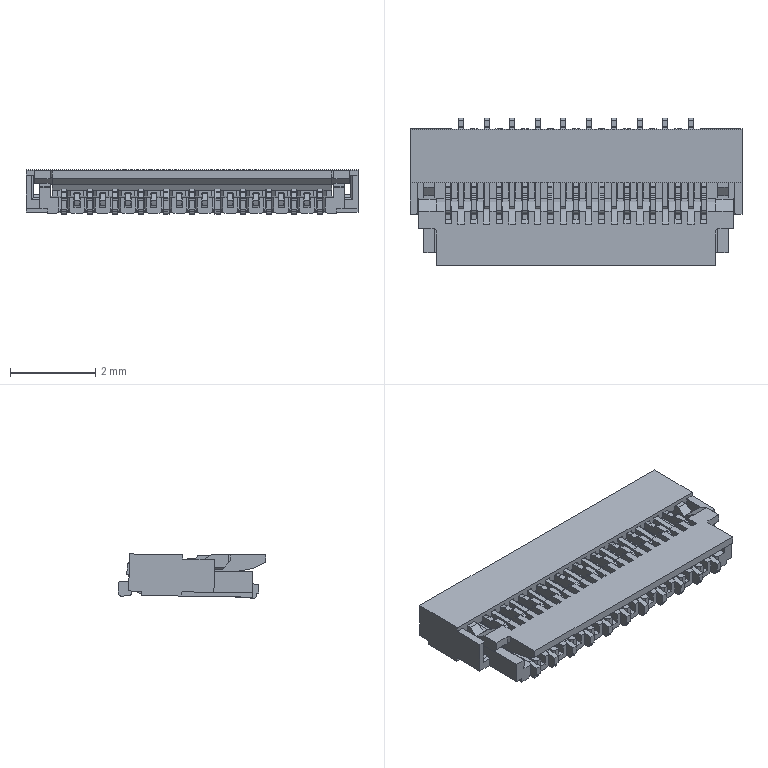Part | Creo | 1 solid | 1933 faces | box 7.8 x 3.471 x 1.037 mm | volume 14.743 mm3 | plane 1279 | cylinder 652 | cone 2 | commonest cylinder face diameters 0.1 x302 0.12 x73 0.2 x73 0.08 x53 0.11 x33 0.6 x30